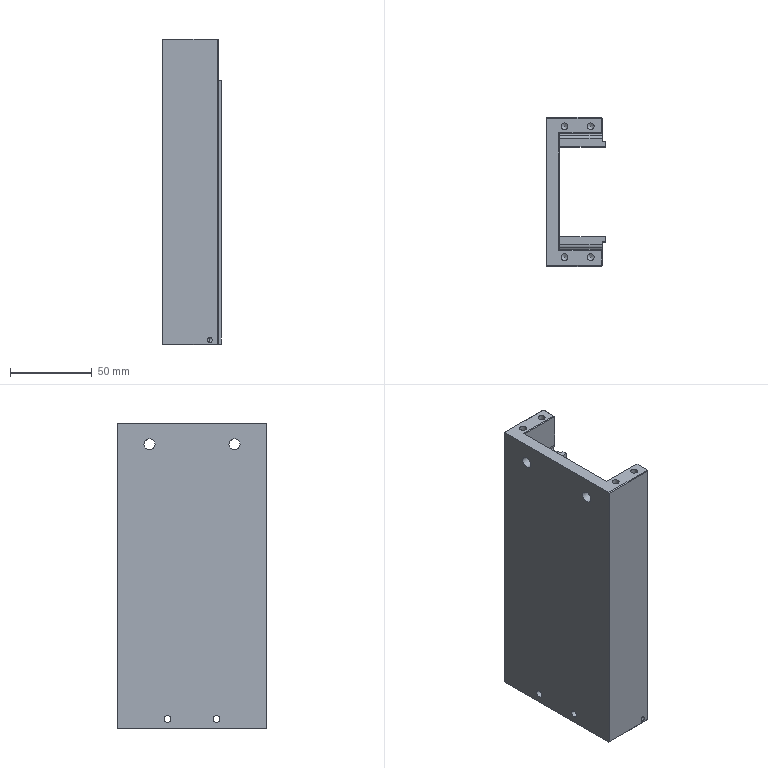Part | 1 solid | 91 faces | box 36 x 91 x 187 mm | volume 300248 mm3 | plane 45 | cylinder 30 | cone 16 | commonest cylinder face diameters 2.5 x10 3 x8 4.2 x6 5 x4 6.8 x2